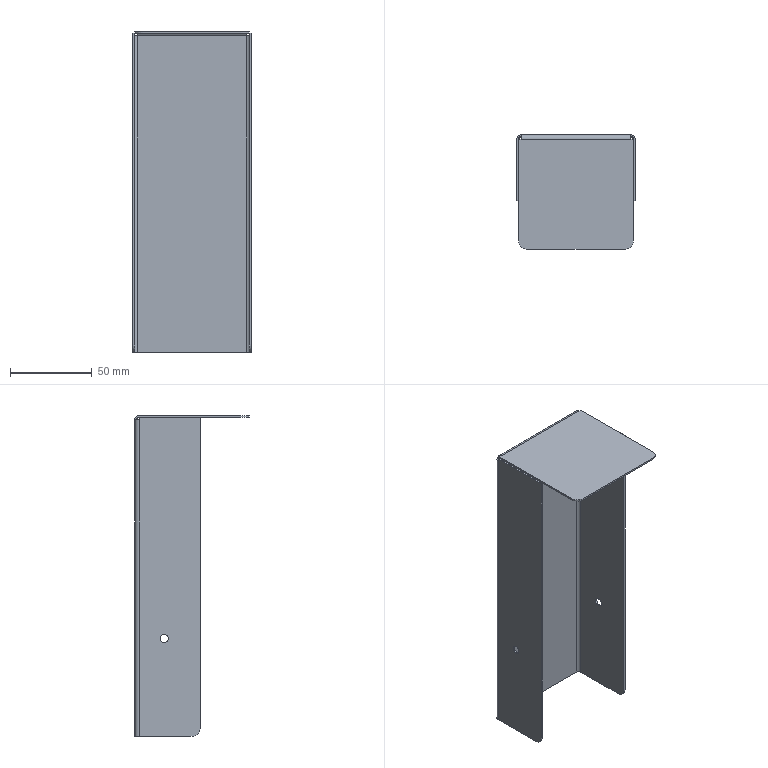Part | NX | 1 solid | 38 faces | box 72.4 x 70 x 196.5 mm | volume 33824 mm3 | plane 24 | cylinder 14 | commonest cylinder face diameters 5 x4 10 x4 3.2 x3 5.2 x3
STEP:
#1=CARTESIAN_POINT('',(-126.2,177.2,177.629));
#2=VERTEX_POINT('',#1);
#3=CARTESIAN_POINT('',(-126.2,214.6,177.629));
#4=VERTEX_POINT('',#3);
#5=CARTESIAN_POINT('',(-126.2,216.2,177.629));
#6=DIRECTION('',(0.,1.,0.));
#7=VECTOR('',#6,1000.);
#8=LINE('',#5,#7);
#9=EDGE_CURVE('',#2,#4,#8,.T.);
#10=ORIENTED_EDGE('',*,*,#9,.T.);
#11=CARTESIAN_POINT('',(-126.2,214.6,176.1));
#12=VERTEX_POINT('',#11);
#13=CARTESIAN_POINT('',(-126.2,214.6,70.628));
#14=DIRECTION('',(0.,0.,-1.));
#15=VECTOR('',#14,1000.);
#16=LINE('',#13,#15);
#17=EDGE_CURVE('',#4,#12,#16,.T.);
#18=ORIENTED_EDGE('',*,*,#17,.T.);
#19=CARTESIAN_POINT('',(-126.2,214.6,-17.8));
#20=VERTEX_POINT('',#19);
#21=CARTESIAN_POINT('',(-126.2,214.6,70.628));
#22=DIRECTION('',(0.,0.,-1.));
#23=VECTOR('',#22,1000.);
#24=LINE('',#21,#23);
#25=EDGE_CURVE('',#12,#20,#24,.T.);
#26=ORIENTED_EDGE('',*,*,#25,.T.);
#27=CARTESIAN_POINT('',(-126.2,182.2,-17.8));
#28=VERTEX_POINT('',#27);
#29=CARTESIAN_POINT('',(-126.2,177.2,-17.8));
#30=DIRECTION('',(0.,1.,0.));
#31=VECTOR('',#30,1000.);
#32=LINE('',#29,#31);
#33=EDGE_CURVE('',#28,#20,#32,.T.);
#34=ORIENTED_EDGE('',*,*,#33,.F.);
#35=CARTESIAN_POINT('',(-126.2,177.2,-12.8));
#36=VERTEX_POINT('',#35);
#37=CARTESIAN_POINT('',(-126.2,182.2,-12.8));
#38=DIRECTION('',(1.,0.,0.));
#39=DIRECTION('',(0.,0.,1.));
#40=AXIS2_PLACEMENT_3D('',#37,#38,#39);
#41=CIRCLE('',#40,5.);
#42=EDGE_CURVE('',#36,#28,#41,.T.);
#43=ORIENTED_EDGE('',*,*,#42,.F.);
#44=CARTESIAN_POINT('',(-126.2,177.2,70.628));
#45=DIRECTION('',(0.,0.,-1.));
#46=VECTOR('',#45,1000.);
#47=LINE('',#44,#46);
#48=EDGE_CURVE('',#2,#36,#47,.T.);
#49=ORIENTED_EDGE('',*,*,#48,.F.);
#50=EDGE_LOOP('',(#10,#18,#26,#34,#43,#49));
#51=FACE_BOUND('',#50,.T.);
#52=CARTESIAN_POINT('',(-126.2,201.7,42.2));
#53=VERTEX_POINT('',#52);
#54=CARTESIAN_POINT('',(-126.2,196.7,42.2));
#55=VERTEX_POINT('',#54);
#56=CARTESIAN_POINT('',(-126.2,199.2,42.2));
#57=DIRECTION('',(1.,0.,0.));
#58=DIRECTION('',(0.,-1.,0.));
#59=AXIS2_PLACEMENT_3D('',#56,#57,#58);
#60=CIRCLE('',#59,2.5);
#61=EDGE_CURVE('',#53,#55,#60,.T.);
#62=ORIENTED_EDGE('',*,*,#61,.T.);
#63=CARTESIAN_POINT('',(-126.2,199.2,42.2));
#64=DIRECTION('',(1.,0.,0.));
#65=DIRECTION('',(0.,-1.,0.));
#66=AXIS2_PLACEMENT_3D('',#63,#64,#65);
#67=CIRCLE('',#66,2.5);
#68=EDGE_CURVE('',#55,#53,#67,.T.);
#69=ORIENTED_EDGE('',*,*,#68,.T.);
#70=EDGE_LOOP('',(#62,#69));
#71=FACE_BOUND('',#70,.T.);
#72=CARTESIAN_POINT('',(-126.2,252.682,70.628));
#73=DIRECTION('',(-1.,0.,0.));
#74=DIRECTION('',(0.,0.,1.));
#75=AXIS2_PLACEMENT_3D('',#72,#73,#74);
#76=PLANE('',#75);
#77=ADVANCED_FACE('',(#51,#71),#76,.T.);
#78=CARTESIAN_POINT('',(-123.6,217.2,176.1));
#79=VERTEX_POINT('',#78);
#80=CARTESIAN_POINT('',(-123.6,217.2,-17.8));
#81=VERTEX_POINT('',#80);
#82=CARTESIAN_POINT('',(-123.6,217.2,70.628));
#83=DIRECTION('',(0.,0.,-1.));
#84=VECTOR('',#83,1000.);
#85=LINE('',#82,#84);
#86=EDGE_CURVE('',#79,#81,#85,.T.);
#87=ORIENTED_EDGE('',*,*,#86,.F.);
#88=CARTESIAN_POINT('',(-56.4,217.2,176.1));
#89=VERTEX_POINT('',#88);
#90=CARTESIAN_POINT('',(-88.618,217.2,176.1));
#91=DIRECTION('',(-1.,0.,0.));
#92=VECTOR('',#91,1000.);
#93=LINE('',#90,#92);
#94=EDGE_CURVE('',#89,#79,#93,.T.);
#95=ORIENTED_EDGE('',*,*,#94,.F.);
#96=CARTESIAN_POINT('',(-56.4,217.2,-17.8));
#97=VERTEX_POINT('',#96);
#98=CARTESIAN_POINT('',(-56.4,217.2,70.628));
#99=DIRECTION('',(0.,0.,1.));
#100=VECTOR('',#99,1000.);
#101=LINE('',#98,#100);
#102=EDGE_CURVE('',#97,#89,#101,.T.);
#103=ORIENTED_EDGE('',*,*,#102,.F.);
#104=CARTESIAN_POINT('',(-53.8,217.2,-17.8));
#105=DIRECTION('',(1.,0.,0.));
#106=VECTOR('',#105,1000.);
#107=LINE('',#104,#106);
#108=EDGE_CURVE('',#81,#97,#107,.T.);
#109=ORIENTED_EDGE('',*,*,#108,.F.);
#110=EDGE_LOOP('',(#87,#95,#103,#109));
#111=FACE_BOUND('',#110,.T.);
#112=CARTESIAN_POINT('',(-88.618,217.2,70.628));
#113=DIRECTION('',(0.,1.,0.));
#114=DIRECTION('',(0.,0.,-1.));
#115=AXIS2_PLACEMENT_3D('',#112,#113,#114);
#116=PLANE('',#115);
#117=ADVANCED_FACE('',(#111),#116,.T.);
#118=ORIENTED_EDGE('',*,*,#25,.F.);
#119=CARTESIAN_POINT('',(-123.6,214.6,176.1));
#120=DIRECTION('',(0.,0.,-1.));
#121=DIRECTION('',(-1.,0.,0.));
#122=AXIS2_PLACEMENT_3D('',#119,#120,#121);
#123=CIRCLE('',#122,2.6);
#124=EDGE_CURVE('',#12,#79,#123,.T.);
#125=ORIENTED_EDGE('',*,*,#124,.T.);
#126=ORIENTED_EDGE('',*,*,#86,.T.);
#127=CARTESIAN_POINT('',(-123.6,214.6,-17.8));
#128=DIRECTION('',(0.,0.,-1.));
#129=DIRECTION('',(-1.,0.,0.));
#130=AXIS2_PLACEMENT_3D('',#127,#128,#129);
#131=CIRCLE('',#130,2.6);
#132=EDGE_CURVE('',#20,#81,#131,.T.);
#133=ORIENTED_EDGE('',*,*,#132,.F.);
#134=EDGE_LOOP('',(#118,#125,#126,#133));
#135=FACE_BOUND('',#134,.T.);
#136=CARTESIAN_POINT('',(-123.6,214.6,-17.8));
#137=DIRECTION('',(0.,0.,-1.));
#138=DIRECTION('',(1.,0.,0.));
#139=AXIS2_PLACEMENT_3D('',#136,#137,#138);
#140=CYLINDRICAL_SURFACE('',#139,2.6);
#141=ADVANCED_FACE('',(#135),#140,.T.);
#142=CARTESIAN_POINT('',(-53.8,214.6,176.1));
#143=VERTEX_POINT('',#142);
#144=CARTESIAN_POINT('',(-53.8,214.6,177.629));
#145=VERTEX_POINT('',#144);
#146=CARTESIAN_POINT('',(-53.8,214.6,70.628));
#147=DIRECTION('',(0.,0.,1.));
#148=VECTOR('',#147,1000.);
#149=LINE('',#146,#148);
#150=EDGE_CURVE('',#143,#145,#149,.T.);
#151=ORIENTED_EDGE('',*,*,#150,.F.);
#152=CARTESIAN_POINT('',(-54.8,214.6,176.1));
#153=VERTEX_POINT('',#152);
#154=CARTESIAN_POINT('',(-53.8,214.6,176.1));
#155=DIRECTION('',(-1.,0.,0.));
#156=VECTOR('',#155,1000.);
#157=LINE('',#154,#156);
#158=EDGE_CURVE('',#143,#153,#157,.T.);
#159=ORIENTED_EDGE('',*,*,#158,.T.);
#160=CARTESIAN_POINT('',(-54.8,214.6,177.629));
#161=VERTEX_POINT('',#160);
#162=CARTESIAN_POINT('',(-54.8,214.6,70.628));
#163=DIRECTION('',(0.,0.,1.));
#164=VECTOR('',#163,1000.);
#165=LINE('',#162,#164);
#166=EDGE_CURVE('',#153,#161,#165,.T.);
#167=ORIENTED_EDGE('',*,*,#166,.T.);
#168=CARTESIAN_POINT('',(-54.8,214.6,177.629));
#169=DIRECTION('',(-1.,0.,0.));
#170=VECTOR('',#169,1000.);
#171=LINE('',#168,#170);
#172=EDGE_CURVE('',#145,#161,#171,.T.);
#173=ORIENTED_EDGE('',*,*,#172,.F.);
#174=EDGE_LOOP('',(#151,#159,#167,#173));
#175=FACE_BOUND('',#174,.T.);
#176=CARTESIAN_POINT('',(-53.8,214.6,176.1));
#177=DIRECTION('',(0.,1.,0.));
#178=DIRECTION('',(0.,0.,-1.));
#179=AXIS2_PLACEMENT_3D('',#176,#177,#178);
#180=PLANE('',#179);
#181=ADVANCED_FACE('',(#175),#180,.T.);
#182=CARTESIAN_POINT('',(-53.8,177.2,177.629));
#183=VERTEX_POINT('',#182);
#184=CARTESIAN_POINT('',(-53.8,216.2,177.629));
#185=DIRECTION('',(0.,-1.,0.));
#186=VECTOR('',#185,1000.);
#187=LINE('',#184,#186);
#188=EDGE_CURVE('',#145,#183,#187,.T.);
#189=ORIENTED_EDGE('',*,*,#188,.T.);
#190=CARTESIAN_POINT('',(-53.8,177.2,-12.8));
#191=VERTEX_POINT('',#190);
#192=CARTESIAN_POINT('',(-53.8,177.2,70.628));
#193=DIRECTION('',(0.,0.,1.));
#194=VECTOR('',#193,1000.);
#195=LINE('',#192,#194);
#196=EDGE_CURVE('',#191,#183,#195,.T.);
#197=ORIENTED_EDGE('',*,*,#196,.F.);
#198=CARTESIAN_POINT('',(-53.8,182.2,-17.8));
#199=VERTEX_POINT('',#198);
#200=CARTESIAN_POINT('',(-53.8,182.2,-12.8));
#201=DIRECTION('',(-1.,0.,0.));
#202=DIRECTION('',(0.,0.,-1.));
#203=AXIS2_PLACEMENT_3D('',#200,#201,#202);
#204=CIRCLE('',#203,5.);
#205=EDGE_CURVE('',#199,#191,#204,.T.);
#206=ORIENTED_EDGE('',*,*,#205,.F.);
#207=CARTESIAN_POINT('',(-53.8,214.6,-17.8));
#208=VERTEX_POINT('',#207);
#209=CARTESIAN_POINT('',(-53.8,215.1,-17.8));
#210=DIRECTION('',(0.,-1.,0.));
#211=VECTOR('',#210,1000.);
#212=LINE('',#209,#211);
#213=EDGE_CURVE('',#208,#199,#212,.T.);
#214=ORIENTED_EDGE('',*,*,#213,.F.);
#215=CARTESIAN_POINT('',(-53.8,214.6,70.628));
#216=DIRECTION('',(0.,0.,1.));
#217=VECTOR('',#216,1000.);
#218=LINE('',#215,#217);
#219=EDGE_CURVE('',#208,#143,#218,.T.);
#220=ORIENTED_EDGE('',*,*,#219,.T.);
#221=ORIENTED_EDGE('',*,*,#150,.T.);
#222=EDGE_LOOP('',(#189,#197,#206,#214,#220,#221));
#223=FACE_BOUND('',#222,.T.);
#224=CARTESIAN_POINT('',(-53.8,201.7,42.2));
#225=VERTEX_POINT('',#224);
#226=CARTESIAN_POINT('',(-53.8,196.7,42.2));
#227=VERTEX_POINT('',#226);
#228=CARTESIAN_POINT('',(-53.8,199.2,42.2));
#229=DIRECTION('',(1.,0.,0.));
#230=DIRECTION('',(0.,-1.,0.));
#231=AXIS2_PLACEMENT_3D('',#228,#229,#230);
#232=CIRCLE('',#231,2.5);
#233=EDGE_CURVE('',#225,#227,#232,.T.);
#234=ORIENTED_EDGE('',*,*,#233,.F.);
#235=CARTESIAN_POINT('',(-53.8,199.2,42.2));
#236=DIRECTION('',(1.,0.,0.));
#237=DIRECTION('',(0.,-1.,0.));
#238=AXIS2_PLACEMENT_3D('',#235,#236,#237);
#239=CIRCLE('',#238,2.5);
#240=EDGE_CURVE('',#227,#225,#239,.T.);
#241=ORIENTED_EDGE('',*,*,#240,.F.);
#242=EDGE_LOOP('',(#234,#241));
#243=FACE_BOUND('',#242,.T.);
#244=CARTESIAN_POINT('',(-53.8,249.918,70.628));
#245=DIRECTION('',(1.,0.,0.));
#246=DIRECTION('',(0.,1.,0.));
#247=AXIS2_PLACEMENT_3D('',#244,#245,#246);
#248=PLANE('',#247);
#249=ADVANCED_FACE('',(#223,#243),#248,.T.);
#250=CARTESIAN_POINT('',(-56.4,214.6,176.1));
#251=DIRECTION('',(0.,0.,-1.));
#252=DIRECTION('',(0.,1.,0.));
#253=AXIS2_PLACEMENT_3D('',#250,#251,#252);
#254=CIRCLE('',#253,2.6);
#255=EDGE_CURVE('',#89,#143,#254,.T.);
#256=ORIENTED_EDGE('',*,*,#255,.T.);
#257=ORIENTED_EDGE('',*,*,#219,.F.);
#258=CARTESIAN_POINT('',(-56.4,214.6,-17.8));
#259=DIRECTION('',(0.,0.,-1.));
#260=DIRECTION('',(0.,1.,0.));
#261=AXIS2_PLACEMENT_3D('',#258,#259,#260);
#262=CIRCLE('',#261,2.6);
#263=EDGE_CURVE('',#97,#208,#262,.T.);
#264=ORIENTED_EDGE('',*,*,#263,.F.);
#265=ORIENTED_EDGE('',*,*,#102,.T.);
#266=EDGE_LOOP('',(#256,#257,#264,#265));
#267=FACE_BOUND('',#266,.T.);
#268=CARTESIAN_POINT('',(-56.4,214.6,176.1));
#269=DIRECTION('',(0.,0.,1.));
#270=DIRECTION('',(-1.,0.,0.));
#271=AXIS2_PLACEMENT_3D('',#268,#269,#270);
#272=CYLINDRICAL_SURFACE('',#271,2.6);
#273=ADVANCED_FACE('',(#267),#272,.T.);
#274=CARTESIAN_POINT('',(-123.6,214.6,178.7));
#275=VERTEX_POINT('',#274);
#276=CARTESIAN_POINT('',(-123.6,214.6,176.1));
#277=DIRECTION('',(1.,0.,0.));
#278=DIRECTION('',(0.,1.,0.));
#279=AXIS2_PLACEMENT_3D('',#276,#277,#278);
#280=CIRCLE('',#279,2.6);
#281=EDGE_CURVE('',#79,#275,#280,.T.);
#282=ORIENTED_EDGE('',*,*,#281,.F.);
#283=CARTESIAN_POINT('',(-123.6,216.2,176.1));
#284=VERTEX_POINT('',#283);
#285=CARTESIAN_POINT('',(-123.6,217.2,176.1));
#286=DIRECTION('',(0.,-1.,0.));
#287=VECTOR('',#286,1000.);
#288=LINE('',#285,#287);
#289=EDGE_CURVE('',#79,#284,#288,.T.);
#290=ORIENTED_EDGE('',*,*,#289,.T.);
#291=CARTESIAN_POINT('',(-123.6,214.6,177.7));
#292=VERTEX_POINT('',#291);
#293=CARTESIAN_POINT('',(-123.6,214.6,176.1));
#294=DIRECTION('',(-1.,0.,0.));
#295=DIRECTION('',(0.,0.,1.));
#296=AXIS2_PLACEMENT_3D('',#293,#294,#295);
#297=CIRCLE('',#296,1.6);
#298=EDGE_CURVE('',#292,#284,#297,.T.);
#299=ORIENTED_EDGE('',*,*,#298,.F.);
#300=CARTESIAN_POINT('',(-123.6,214.6,178.7));
#301=DIRECTION('',(0.,0.,-1.));
#302=VECTOR('',#301,1000.);
#303=LINE('',#300,#302);
#304=EDGE_CURVE('',#275,#292,#303,.T.);
#305=ORIENTED_EDGE('',*,*,#304,.F.);
#306=EDGE_LOOP('',(#282,#290,#299,#305));
#307=FACE_BOUND('',#306,.T.);
#308=CARTESIAN_POINT('',(-123.6,214.6,176.1));
#309=DIRECTION('',(1.,0.,0.));
#310=DIRECTION('',(0.,1.,0.));
#311=AXIS2_PLACEMENT_3D('',#308,#309,#310);
#312=PLANE('',#311);
#313=ADVANCED_FACE('',(#307),#312,.F.);
#314=ORIENTED_EDGE('',*,*,#94,.T.);
#315=ORIENTED_EDGE('',*,*,#281,.T.);
#316=CARTESIAN_POINT('',(-56.4,214.6,178.7));
#317=VERTEX_POINT('',#316);
#318=CARTESIAN_POINT('',(-88.618,214.6,178.7));
#319=DIRECTION('',(-1.,0.,0.));
#320=VECTOR('',#319,1000.);
#321=LINE('',#318,#320);
#322=EDGE_CURVE('',#317,#275,#321,.T.);
#323=ORIENTED_EDGE('',*,*,#322,.F.);
#324=CARTESIAN_POINT('',(-56.4,214.6,176.1));
#325=DIRECTION('',(-1.,0.,0.));
#326=DIRECTION('',(0.,0.,1.));
#327=AXIS2_PLACEMENT_3D('',#324,#325,#326);
#328=CIRCLE('',#327,2.6);
#329=EDGE_CURVE('',#317,#89,#328,.T.);
#330=ORIENTED_EDGE('',*,*,#329,.T.);
#331=EDGE_LOOP('',(#314,#315,#323,#330));
#332=FACE_BOUND('',#331,.T.);
#333=CARTESIAN_POINT('',(-123.6,214.6,176.1));
#334=DIRECTION('',(-1.,0.,0.));
#335=DIRECTION('',(0.,0.,-1.));
#336=AXIS2_PLACEMENT_3D('',#333,#334,#335);
#337=CYLINDRICAL_SURFACE('',#336,2.6);
#338=ADVANCED_FACE('',(#332),#337,.T.);
#339=ORIENTED_EDGE('',*,*,#322,.T.);
#340=CARTESIAN_POINT('',(-125.129,214.6,178.7));
#341=VERTEX_POINT('',#340);
#342=CARTESIAN_POINT('',(-88.618,214.6,178.7));
#343=DIRECTION('',(-1.,0.,0.));
#344=VECTOR('',#343,1000.);
#345=LINE('',#342,#344);
#346=EDGE_CURVE('',#275,#341,#345,.T.);
#347=ORIENTED_EDGE('',*,*,#346,.T.);
#348=CARTESIAN_POINT('',(-125.129,152.2,178.7));
#349=VERTEX_POINT('',#348);
#350=CARTESIAN_POINT('',(-125.129,216.2,178.7));
#351=DIRECTION('',(0.,1.,0.));
#352=VECTOR('',#351,1000.);
#353=LINE('',#350,#352);
#354=EDGE_CURVE('',#349,#341,#353,.T.);
#355=ORIENTED_EDGE('',*,*,#354,.F.);
#356=CARTESIAN_POINT('',(-120.129,147.2,178.7));
#357=VERTEX_POINT('',#356);
#358=CARTESIAN_POINT('',(-120.129,152.2,178.7));
#359=DIRECTION('',(0.,0.,1.));
#360=DIRECTION('',(-1.,0.,0.));
#361=AXIS2_PLACEMENT_3D('',#358,#359,#360);
#362=CIRCLE('',#361,5.);
#363=EDGE_CURVE('',#349,#357,#362,.T.);
#364=ORIENTED_EDGE('',*,*,#363,.T.);
#365=CARTESIAN_POINT('',(-59.871,147.2,178.7));
#366=VERTEX_POINT('',#365);
#367=CARTESIAN_POINT('',(-88.618,147.2,178.7));
#368=DIRECTION('',(1.,0.,0.));
#369=VECTOR('',#368,1000.);
#370=LINE('',#367,#369);
#371=EDGE_CURVE('',#357,#366,#370,.T.);
#372=ORIENTED_EDGE('',*,*,#371,.T.);
#373=CARTESIAN_POINT('',(-54.871,152.2,178.7));
#374=VERTEX_POINT('',#373);
#375=CARTESIAN_POINT('',(-59.871,152.2,178.7));
#376=DIRECTION('',(0.,0.,-1.));
#377=DIRECTION('',(1.,0.,0.));
#378=AXIS2_PLACEMENT_3D('',#375,#376,#377);
#379=CIRCLE('',#378,5.);
#380=EDGE_CURVE('',#374,#366,#379,.T.);
#381=ORIENTED_EDGE('',*,*,#380,.F.);
#382=CARTESIAN_POINT('',(-54.871,214.6,178.7));
#383=VERTEX_POINT('',#382);
#384=CARTESIAN_POINT('',(-54.871,216.2,178.7));
#385=DIRECTION('',(0.,-1.,0.));
#386=VECTOR('',#385,1000.);
#387=LINE('',#384,#386);
#388=EDGE_CURVE('',#383,#374,#387,.T.);
#389=ORIENTED_EDGE('',*,*,#388,.F.);
#390=CARTESIAN_POINT('',(-88.618,214.6,178.7));
#391=DIRECTION('',(-1.,0.,0.));
#392=VECTOR('',#391,1000.);
#393=LINE('',#390,#392);
#394=EDGE_CURVE('',#383,#317,#393,.T.);
#395=ORIENTED_EDGE('',*,*,#394,.T.);
#396=EDGE_LOOP('',(#339,#347,#355,#364,#372,#381,#389,#395));
#397=FACE_BOUND('',#396,.T.);
#398=CARTESIAN_POINT('',(-88.618,323.172,178.7));
#399=DIRECTION('',(0.,0.,1.));
#400=DIRECTION('',(0.,-1.,0.));
#401=AXIS2_PLACEMENT_3D('',#398,#399,#400);
#402=PLANE('',#401);
#403=ADVANCED_FACE('',(#397),#402,.T.);
#404=ORIENTED_EDGE('',*,*,#48,.T.);
#405=CARTESIAN_POINT('',(-125.2,177.2,-12.8));
#406=VERTEX_POINT('',#405);
#407=CARTESIAN_POINT('',(-88.618,177.2,-12.8));
#408=DIRECTION('',(1.,0.,0.));
#409=VECTOR('',#408,1000.);
#410=LINE('',#407,#409);
#411=EDGE_CURVE('',#36,#406,#410,.T.);
#412=ORIENTED_EDGE('',*,*,#411,.T.);
#413=CARTESIAN_POINT('',(-125.2,177.2,177.629));
#414=VERTEX_POINT('',#413);
#415=CARTESIAN_POINT('',(-125.2,177.2,70.628));
#416=DIRECTION('',(0.,0.,-1.));
#417=VECTOR('',#416,1000.);
#418=LINE('',#415,#417);
#419=EDGE_CURVE('',#414,#406,#418,.T.);
#420=ORIENTED_EDGE('',*,*,#419,.F.);
#421=CARTESIAN_POINT('',(-88.618,177.2,177.629));
#422=DIRECTION('',(-1.,0.,0.));
#423=VECTOR('',#422,1000.);
#424=LINE('',#421,#423);
#425=EDGE_CURVE('',#414,#2,#424,.T.);
#426=ORIENTED_EDGE('',*,*,#425,.T.);
#427=EDGE_LOOP('',(#404,#412,#420,#426));
#428=FACE_BOUND('',#427,.T.);
#429=CARTESIAN_POINT('',(-126.2,177.2,-17.8));
#430=DIRECTION('',(0.,-1.,0.));
#431=DIRECTION('',(0.,0.,-1.));
#432=AXIS2_PLACEMENT_3D('',#429,#430,#431);
#433=PLANE('',#432);
#434=ADVANCED_FACE('',(#428),#433,.T.);
#435=CARTESIAN_POINT('',(-125.2,214.6,176.1));
#436=VERTEX_POINT('',#435);
#437=CARTESIAN_POINT('',(-125.2,214.6,-17.8));
#438=VERTEX_POINT('',#437);
#439=CARTESIAN_POINT('',(-125.2,214.6,70.628));
#440=DIRECTION('',(0.,0.,-1.));
#441=VECTOR('',#440,1000.);
#442=LINE('',#439,#441);
#443=EDGE_CURVE('',#436,#438,#442,.T.);
#444=ORIENTED_EDGE('',*,*,#443,.F.);
#445=CARTESIAN_POINT('',(-125.2,214.6,177.629));
#446=VERTEX_POINT('',#445);
#447=CARTESIAN_POINT('',(-125.2,214.6,70.628));
#448=DIRECTION('',(0.,0.,-1.));
#449=VECTOR('',#448,1000.);
#450=LINE('',#447,#449);
#451=EDGE_CURVE('',#446,#436,#450,.T.);
#452=ORIENTED_EDGE('',*,*,#451,.F.);
#453=CARTESIAN_POINT('',(-125.2,216.2,177.629));
#454=DIRECTION('',(0.,1.,0.));
#455=VECTOR('',#454,1000.);
#456=LINE('',#453,#455);
#457=EDGE_CURVE('',#414,#446,#456,.T.);
#458=ORIENTED_EDGE('',*,*,#457,.F.);
#459=ORIENTED_EDGE('',*,*,#419,.T.);
#460=CARTESIAN_POINT('',(-125.2,182.2,-17.8));
#461=VERTEX_POINT('',#460);
#462=CARTESIAN_POINT('',(-125.2,182.2,-12.8));
#463=DIRECTION('',(1.,0.,0.));
#464=DIRECTION('',(0.,0.,1.));
#465=AXIS2_PLACEMENT_3D('',#462,#463,#464);
#466=CIRCLE('',#465,5.);
#467=EDGE_CURVE('',#406,#461,#466,.T.);
#468=ORIENTED_EDGE('',*,*,#467,.T.);
#469=CARTESIAN_POINT('',(-125.2,177.2,-17.8));
#470=DIRECTION('',(0.,1.,0.));
#471=VECTOR('',#470,1000.);
#472=LINE('',#469,#471);
#473=EDGE_CURVE('',#461,#438,#472,.T.);
#474=ORIENTED_EDGE('',*,*,#473,.T.);
#475=EDGE_LOOP('',(#444,#452,#458,#459,#468,#474));
#476=FACE_BOUND('',#475,.T.);
#477=CARTESIAN_POINT('',(-125.2,201.7,42.2));
#478=VERTEX_POINT('',#477);
#479=CARTESIAN_POINT('',(-125.2,196.7,42.2));
#480=VERTEX_POINT('',#479);
#481=CARTESIAN_POINT('',(-125.2,199.2,42.2));
#482=DIRECTION('',(1.,0.,0.));
#483=DIRECTION('',(0.,-1.,0.));
#484=AXIS2_PLACEMENT_3D('',#481,#482,#483);
#485=CIRCLE('',#484,2.5);
#486=EDGE_CURVE('',#478,#480,#485,.T.);
#487=ORIENTED_EDGE('',*,*,#486,.F.);
#488=CARTESIAN_POINT('',(-125.2,199.2,42.2));
#489=DIRECTION('',(1.,0.,0.));
#490=DIRECTION('',(0.,-1.,0.));
#491=AXIS2_PLACEMENT_3D('',#488,#489,#490);
#492=CIRCLE('',#491,2.5);
#493=EDGE_CURVE('',#480,#478,#492,.T.);
#494=ORIENTED_EDGE('',*,*,#493,.F.);
#495=EDGE_LOOP('',(#487,#494));
#496=FACE_BOUND('',#495,.T.);
#497=CARTESIAN_POINT('',(-125.2,215.1,175.2));
#498=DIRECTION('',(-1.,0.,0.));
#499=DIRECTION('',(0.,0.,1.));
#500=AXIS2_PLACEMENT_3D('',#497,#498,#499);
#501=PLANE('',#500);
#502=ADVANCED_FACE('',(#476,#496),#501,.F.);
#503=CARTESIAN_POINT('',(-123.6,216.2,-17.8));
#504=VERTEX_POINT('',#503);
#505=CARTESIAN_POINT('',(-123.6,216.2,70.628));
#506=DIRECTION('',(0.,0.,-1.));
#507=VECTOR('',#506,1000.);
#508=LINE('',#505,#507);
#509=EDGE_CURVE('',#284,#504,#508,.T.);
#510=ORIENTED_EDGE('',*,*,#509,.F.);
#511=CARTESIAN_POINT('',(-123.6,214.6,176.1));
#512=DIRECTION('',(0.,0.,1.));
#513=DIRECTION('',(0.,1.,0.));
#514=AXIS2_PLACEMENT_3D('',#511,#512,#513);
#515=CIRCLE('',#514,1.6);
#516=EDGE_CURVE('',#284,#436,#515,.T.);
#517=ORIENTED_EDGE('',*,*,#516,.T.);
#518=ORIENTED_EDGE('',*,*,#443,.T.);
#519=CARTESIAN_POINT('',(-123.6,214.6,-17.8));
#520=DIRECTION('',(0.,0.,-1.));
#521=DIRECTION('',(-1.,0.,0.));
#522=AXIS2_PLACEMENT_3D('',#519,#520,#521);
#523=CIRCLE('',#522,1.6);
#524=EDGE_CURVE('',#438,#504,#523,.T.);
#525=ORIENTED_EDGE('',*,*,#524,.T.);
#526=EDGE_LOOP('',(#510,#517,#518,#525));
#527=FACE_BOUND('',#526,.T.);
#528=CARTESIAN_POINT('',(-123.6,214.6,-17.8));
#529=DIRECTION('',(0.,0.,-1.));
#530=DIRECTION('',(1.,0.,0.));
#531=AXIS2_PLACEMENT_3D('',#528,#529,#530);
#532=CYLINDRICAL_SURFACE('',#531,1.6);
#533=ADVANCED_FACE('',(#527),#532,.F.);
#534=ORIENTED_EDGE('',*,*,#61,.F.);
#535=CARTESIAN_POINT('',(-133.44,201.7,42.2));
#536=DIRECTION('',(1.,0.,0.));
#537=VECTOR('',#536,1000.);
#538=LINE('',#535,#537);
#539=EDGE_CURVE('',#478,#53,#538,.F.);
#540=ORIENTED_EDGE('',*,*,#539,.F.);
#541=ORIENTED_EDGE('',*,*,#486,.T.);
#542=CARTESIAN_POINT('',(-133.44,196.7,42.2));
#543=DIRECTION('',(1.,0.,0.));
#544=VECTOR('',#543,1000.);
#545=LINE('',#542,#544);
#546=EDGE_CURVE('',#480,#55,#545,.F.);
#547=ORIENTED_EDGE('',*,*,#546,.T.);
#548=EDGE_LOOP('',(#534,#540,#541,#547));
#549=FACE_BOUND('',#548,.T.);
#550=CARTESIAN_POINT('',(-133.44,199.2,42.2));
#551=DIRECTION('',(1.,0.,0.));
#552=DIRECTION('',(0.,-1.,0.));
#553=AXIS2_PLACEMENT_3D('',#550,#551,#552);
#554=CYLINDRICAL_SURFACE('',#553,2.5);
#555=ADVANCED_FACE('',(#549),#554,.F.);
#556=ORIENTED_EDGE('',*,*,#546,.F.);
#557=ORIENTED_EDGE('',*,*,#493,.T.);
#558=ORIENTED_EDGE('',*,*,#539,.T.);
#559=ORIENTED_EDGE('',*,*,#68,.F.);
#560=EDGE_LOOP('',(#556,#557,#558,#559));
#561=FACE_BOUND('',#560,.T.);
#562=CARTESIAN_POINT('',(-133.44,199.2,42.2));
#563=DIRECTION('',(1.,0.,0.));
#564=DIRECTION('',(0.,-1.,0.));
#565=AXIS2_PLACEMENT_3D('',#562,#563,#564);
#566=CYLINDRICAL_SURFACE('',#565,2.5);
#567=ADVANCED_FACE('',(#561),#566,.F.);
#568=CARTESIAN_POINT('',(-54.8,214.6,-17.8));
#569=VERTEX_POINT('',#568);
#570=CARTESIAN_POINT('',(-54.8,182.2,-17.8));
#571=VERTEX_POINT('',#570);
#572=CARTESIAN_POINT('',(-54.8,215.1,-17.8));
#573=DIRECTION('',(0.,-1.,0.));
#574=VECTOR('',#573,1000.);
#575=LINE('',#572,#574);
#576=EDGE_CURVE('',#569,#571,#575,.T.);
#577=ORIENTED_EDGE('',*,*,#576,.T.);
#578=CARTESIAN_POINT('',(-54.8,177.2,-12.8));
#579=VERTEX_POINT('',#578);
#580=CARTESIAN_POINT('',(-54.8,182.2,-12.8));
#581=DIRECTION('',(-1.,0.,0.));
#582=DIRECTION('',(0.,0.,-1.));
#583=AXIS2_PLACEMENT_3D('',#580,#581,#582);
#584=CIRCLE('',#583,5.);
#585=EDGE_CURVE('',#571,#579,#584,.T.);
#586=ORIENTED_EDGE('',*,*,#585,.T.);
#587=CARTESIAN_POINT('',(-54.8,177.2,177.629));
#588=VERTEX_POINT('',#587);
#589=CARTESIAN_POINT('',(-54.8,177.2,70.628));
#590=DIRECTION('',(0.,0.,1.));
#591=VECTOR('',#590,1000.);
#592=LINE('',#589,#591);
#593=EDGE_CURVE('',#579,#588,#592,.T.);
#594=ORIENTED_EDGE('',*,*,#593,.T.);
#595=CARTESIAN_POINT('',(-54.8,216.2,177.629));
#596=DIRECTION('',(0.,-1.,0.));
#597=VECTOR('',#596,1000.);
#598=LINE('',#595,#597);
#599=EDGE_CURVE('',#161,#588,#598,.T.);
#600=ORIENTED_EDGE('',*,*,#599,.F.);
#601=ORIENTED_EDGE('',*,*,#166,.F.);
#602=CARTESIAN_POINT('',(-54.8,214.6,70.628));
#603=DIRECTION('',(0.,0.,1.));
#604=VECTOR('',#603,1000.);
#605=LINE('',#602,#604);
#606=EDGE_CURVE('',#569,#153,#605,.T.);
#607=ORIENTED_EDGE('',*,*,#606,.F.);
#608=EDGE_LOOP('',(#577,#586,#594,#600,#601,#607));
#609=FACE_BOUND('',#608,.T.);
#610=CARTESIAN_POINT('',(-54.8,201.7,42.2));
#611=VERTEX_POINT('',#610);
#612=CARTESIAN_POINT('',(-54.8,196.7,42.2));
#613=VERTEX_POINT('',#612);
#614=CARTESIAN_POINT('',(-54.8,199.2,42.2));
#615=DIRECTION('',(1.,0.,0.));
#616=DIRECTION('',(0.,-1.,0.));
#617=AXIS2_PLACEMENT_3D('',#614,#615,#616);
#618=CIRCLE('',#617,2.5);
#619=EDGE_CURVE('',#611,#613,#618,.T.);
#620=ORIENTED_EDGE('',*,*,#619,.T.);
#621=CARTESIAN_POINT('',(-54.8,199.2,42.2));
#622=DIRECTION('',(1.,0.,0.));
#623=DIRECTION('',(0.,-1.,0.));
#624=AXIS2_PLACEMENT_3D('',#621,#622,#623);
#625=CIRCLE('',#624,2.5);
#626=EDGE_CURVE('',#613,#611,#625,.T.);
#627=ORIENTED_EDGE('',*,*,#626,.T.);
#628=EDGE_LOOP('',(#620,#627));
#629=FACE_BOUND('',#628,.T.);
#630=CARTESIAN_POINT('',(-54.8,215.1,-17.8));
#631=DIRECTION('',(1.,0.,0.));
#632=DIRECTION('',(0.,1.,0.));
#633=AXIS2_PLACEMENT_3D('',#630,#631,#632);
#634=PLANE('',#633);
#635=ADVANCED_FACE('',(#609,#629),#634,.F.);
#636=ORIENTED_EDGE('',*,*,#196,.T.);
#637=CARTESIAN_POINT('',(-88.618,177.2,177.629));
#638=DIRECTION('',(-1.,0.,0.));
#639=VECTOR('',#638,1000.);
#640=LINE('',#637,#639);
#641=EDGE_CURVE('',#183,#588,#640,.T.);
#642=ORIENTED_EDGE('',*,*,#641,.T.);
#643=ORIENTED_EDGE('',*,*,#593,.F.);
#644=CARTESIAN_POINT('',(-88.618,177.2,-12.8));
#645=DIRECTION('',(-1.,0.,0.));
#646=VECTOR('',#645,1000.);
#647=LINE('',#644,#646);
#648=EDGE_CURVE('',#191,#579,#647,.T.);
#649=ORIENTED_EDGE('',*,*,#648,.F.);
#650=EDGE_LOOP('',(#636,#642,#643,#649));
#651=FACE_BOUND('',#650,.T.);
#652=CARTESIAN_POINT('',(-53.8,177.2,175.2));
#653=DIRECTION('',(0.,-1.,0.));
#654=DIRECTION('',(0.,0.,-1.));
#655=AXIS2_PLACEMENT_3D('',#652,#653,#654);
#656=PLANE('',#655);
#657=ADVANCED_FACE('',(#651),#656,.T.);
#658=CARTESIAN_POINT('',(-125.2,214.6,177.629));
#659=DIRECTION('',(-1.,0.,0.));
#660=VECTOR('',#659,1000.);
#661=LINE('',#658,#660);
#662=EDGE_CURVE('',#446,#4,#661,.T.);
#663=ORIENTED_EDGE('',*,*,#662,.T.);
#664=ORIENTED_EDGE('',*,*,#9,.F.);
#665=ORIENTED_EDGE('',*,*,#425,.F.);
#666=ORIENTED_EDGE('',*,*,#457,.T.);
#667=EDGE_LOOP('',(#663,#664,#665,#666));
#668=FACE_BOUND('',#667,.T.);
#669=CARTESIAN_POINT('',(-125.2,195.9,177.629));
#670=DIRECTION('',(0.,0.,1.));
#671=DIRECTION('',(1.,0.,0.));
#672=AXIS2_PLACEMENT_3D('',#669,#670,#671);
#673=PLANE('',#672);
#674=ADVANCED_FACE('',(#668),#673,.T.);
#675=ORIENTED_EDGE('',*,*,#599,.T.);
#676=ORIENTED_EDGE('',*,*,#641,.F.);
#677=ORIENTED_EDGE('',*,*,#188,.F.);
#678=ORIENTED_EDGE('',*,*,#172,.T.);
#679=EDGE_LOOP('',(#675,#676,#677,#678));
#680=FACE_BOUND('',#679,.T.);
#681=CARTESIAN_POINT('',(-54.8,195.9,177.629));
#682=DIRECTION('',(0.,0.,1.));
#683=DIRECTION('',(1.,0.,0.));
#684=AXIS2_PLACEMENT_3D('',#681,#682,#683);
#685=PLANE('',#684);
#686=ADVANCED_FACE('',(#680),#685,.T.);
#687=CARTESIAN_POINT('',(-56.4,214.6,177.7));
#688=VERTEX_POINT('',#687);
#689=CARTESIAN_POINT('',(-56.4,216.2,176.1));
#690=VERTEX_POINT('',#689);
#691=CARTESIAN_POINT('',(-56.4,214.6,176.1));
#692=DIRECTION('',(-1.,0.,0.));
#693=DIRECTION('',(0.,0.,1.));
#694=AXIS2_PLACEMENT_3D('',#691,#692,#693);
#695=CIRCLE('',#694,1.6);
#696=EDGE_CURVE('',#688,#690,#695,.T.);
#697=ORIENTED_EDGE('',*,*,#696,.F.);
#698=CARTESIAN_POINT('',(-88.618,214.6,177.7));
#699=DIRECTION('',(-1.,0.,0.));
#700=VECTOR('',#699,1000.);
#701=LINE('',#698,#700);
#702=EDGE_CURVE('',#688,#292,#701,.T.);
#703=ORIENTED_EDGE('',*,*,#702,.T.);
#704=ORIENTED_EDGE('',*,*,#298,.T.);
#705=CARTESIAN_POINT('',(-88.618,216.2,176.1));
#706=DIRECTION('',(-1.,0.,0.));
#707=VECTOR('',#706,1000.);
#708=LINE('',#705,#707);
#709=EDGE_CURVE('',#690,#284,#708,.T.);
#710=ORIENTED_EDGE('',*,*,#709,.F.);
#711=EDGE_LOOP('',(#697,#703,#704,#710));
#712=FACE_BOUND('',#711,.T.);
#713=CARTESIAN_POINT('',(-123.6,214.6,176.1));
#714=DIRECTION('',(-1.,0.,0.));
#715=DIRECTION('',(0.,0.,-1.));
#716=AXIS2_PLACEMENT_3D('',#713,#714,#715);
#717=CYLINDRICAL_SURFACE('',#716,1.6);
#718=ADVANCED_FACE('',(#712),#717,.F.);
#719=CARTESIAN_POINT('',(-56.4,214.6,176.1));
#720=DIRECTION('',(0.,0.,1.));
#721=DIRECTION('',(1.,0.,0.));
#722=AXIS2_PLACEMENT_3D('',#719,#720,#721);
#723=CIRCLE('',#722,1.6);
#724=EDGE_CURVE('',#153,#690,#723,.T.);
#725=ORIENTED_EDGE('',*,*,#724,.T.);
#726=CARTESIAN_POINT('',(-56.4,216.2,-17.8));
#727=VERTEX_POINT('',#726);
#728=CARTESIAN_POINT('',(-56.4,216.2,70.628));
#729=DIRECTION('',(0.,0.,1.));
#730=VECTOR('',#729,1000.);
#731=LINE('',#728,#730);
#732=EDGE_CURVE('',#727,#690,#731,.T.);
#733=ORIENTED_EDGE('',*,*,#732,.F.);
#734=CARTESIAN_POINT('',(-56.4,214.6,-17.8));
#735=DIRECTION('',(0.,0.,-1.));
#736=DIRECTION('',(0.,1.,0.));
#737=AXIS2_PLACEMENT_3D('',#734,#735,#736);
#738=CIRCLE('',#737,1.6);
#739=EDGE_CURVE('',#727,#569,#738,.T.);
#740=ORIENTED_EDGE('',*,*,#739,.T.);
#741=ORIENTED_EDGE('',*,*,#606,.T.);
#742=EDGE_LOOP('',(#725,#733,#740,#741));
#743=FACE_BOUND('',#742,.T.);
#744=CARTESIAN_POINT('',(-56.4,214.6,176.1));
#745=DIRECTION('',(0.,0.,1.));
#746=DIRECTION('',(-1.,0.,0.));
#747=AXIS2_PLACEMENT_3D('',#744,#745,#746);
#748=CYLINDRICAL_SURFACE('',#747,1.6);
#749=ADVANCED_FACE('',(#743),#748,.F.);
#750=CARTESIAN_POINT('',(-88.618,182.2,-17.8));
#751=DIRECTION('',(-1.,0.,0.));
#752=VECTOR('',#751,1000.);
#753=LINE('',#750,#752);
#754=EDGE_CURVE('',#199,#571,#753,.T.);
#755=ORIENTED_EDGE('',*,*,#754,.T.);
#756=ORIENTED_EDGE('',*,*,#576,.F.);
#757=ORIENTED_EDGE('',*,*,#739,.F.);
#758=CARTESIAN_POINT('',(-53.8,216.2,-17.8));
#759=DIRECTION('',(1.,0.,0.));
#760=VECTOR('',#759,1000.);
#761=LINE('',#758,#760);
#762=EDGE_CURVE('',#504,#727,#761,.T.);
#763=ORIENTED_EDGE('',*,*,#762,.F.);
#764=ORIENTED_EDGE('',*,*,#524,.F.);
#765=ORIENTED_EDGE('',*,*,#473,.F.);
#766=CARTESIAN_POINT('',(-88.618,182.2,-17.8));
#767=DIRECTION('',(1.,0.,0.));
#768=VECTOR('',#767,1000.);
#769=LINE('',#766,#768);
#770=EDGE_CURVE('',#28,#461,#769,.T.);
#771=ORIENTED_EDGE('',*,*,#770,.F.);
#772=ORIENTED_EDGE('',*,*,#33,.T.);
#773=ORIENTED_EDGE('',*,*,#132,.T.);
#774=ORIENTED_EDGE('',*,*,#108,.T.);
#775=ORIENTED_EDGE('',*,*,#263,.T.);
#776=ORIENTED_EDGE('',*,*,#213,.T.);
#777=EDGE_LOOP('',(#755,#756,#757,#763,#764,#765,#771,#772,#773,#774,#775,#776));
#778=FACE_BOUND('',#777,.T.);
#779=CARTESIAN_POINT('',(-15.9,217.2,-17.8));
#780=DIRECTION('',(0.,0.,-1.));
#781=DIRECTION('',(0.,-1.,0.));
#782=AXIS2_PLACEMENT_3D('',#779,#780,#781);
#783=PLANE('',#782);
#784=ADVANCED_FACE('',(#778),#783,.T.);
#785=ORIENTED_EDGE('',*,*,#255,.F.);
#786=CARTESIAN_POINT('',(-56.4,217.2,176.1));
#787=DIRECTION('',(0.,-1.,0.));
#788=VECTOR('',#787,1000.);
#789=LINE('',#786,#788);
#790=EDGE_CURVE('',#89,#690,#789,.T.);
#791=ORIENTED_EDGE('',*,*,#790,.T.);
#792=ORIENTED_EDGE('',*,*,#724,.F.);
#793=ORIENTED_EDGE('',*,*,#158,.F.);
#794=EDGE_LOOP('',(#785,#791,#792,#793));
#795=FACE_BOUND('',#794,.T.);
#796=CARTESIAN_POINT('',(-56.4,214.6,176.1));
#797=DIRECTION('',(0.,0.,-1.));
#798=DIRECTION('',(-1.,0.,0.));
#799=AXIS2_PLACEMENT_3D('',#796,#797,#798);
#800=PLANE('',#799);
#801=ADVANCED_FACE('',(#795),#800,.F.);
#802=CARTESIAN_POINT('',(-125.129,214.6,177.7));
#803=VERTEX_POINT('',#802);
#804=CARTESIAN_POINT('',(-125.129,214.6,177.7));
#805=DIRECTION('',(0.,0.,-1.));
#806=VECTOR('',#805,1000.);
#807=LINE('',#804,#806);
#808=EDGE_CURVE('',#341,#803,#807,.T.);
#809=ORIENTED_EDGE('',*,*,#808,.F.);
#810=ORIENTED_EDGE('',*,*,#346,.F.);
#811=ORIENTED_EDGE('',*,*,#304,.T.);
#812=CARTESIAN_POINT('',(-88.618,214.6,177.7));
#813=DIRECTION('',(-1.,0.,0.));
#814=VECTOR('',#813,1000.);
#815=LINE('',#812,#814);
#816=EDGE_CURVE('',#292,#803,#815,.T.);
#817=ORIENTED_EDGE('',*,*,#816,.T.);
#818=EDGE_LOOP('',(#809,#810,#811,#817));
#819=FACE_BOUND('',#818,.T.);
#820=CARTESIAN_POINT('',(-123.6,214.6,178.7));
#821=DIRECTION('',(0.,1.,0.));
#822=DIRECTION('',(0.,0.,-1.));
#823=AXIS2_PLACEMENT_3D('',#820,#821,#822);
#824=PLANE('',#823);
#825=ADVANCED_FACE('',(#819),#824,.T.);
#826=ORIENTED_EDGE('',*,*,#124,.F.);
#827=CARTESIAN_POINT('',(-126.2,214.6,176.1));
#828=DIRECTION('',(1.,0.,0.));
#829=VECTOR('',#828,1000.);
#830=LINE('',#827,#829);
#831=EDGE_CURVE('',#12,#436,#830,.T.);
#832=ORIENTED_EDGE('',*,*,#831,.T.);
#833=ORIENTED_EDGE('',*,*,#516,.F.);
#834=ORIENTED_EDGE('',*,*,#289,.F.);
#835=EDGE_LOOP('',(#826,#832,#833,#834));
#836=FACE_BOUND('',#835,.T.);
#837=CARTESIAN_POINT('',(-123.6,214.6,176.1));
#838=DIRECTION('',(0.,0.,-1.));
#839=DIRECTION('',(-1.,0.,0.));
#840=AXIS2_PLACEMENT_3D('',#837,#838,#839);
#841=PLANE('',#840);
#842=ADVANCED_FACE('',(#836),#841,.F.);
#843=ORIENTED_EDGE('',*,*,#709,.T.);
#844=ORIENTED_EDGE('',*,*,#509,.T.);
#845=ORIENTED_EDGE('',*,*,#762,.T.);
#846=ORIENTED_EDGE('',*,*,#732,.T.);
#847=EDGE_LOOP('',(#843,#844,#845,#846));
#848=FACE_BOUND('',#847,.T.);
#849=CARTESIAN_POINT('',(-53.8,216.2,-17.8));
#850=DIRECTION('',(0.,1.,0.));
#851=DIRECTION('',(0.,0.,-1.));
#852=AXIS2_PLACEMENT_3D('',#849,#850,#851);
#853=PLANE('',#852);
#854=ADVANCED_FACE('',(#848),#853,.F.);
#855=ORIENTED_EDGE('',*,*,#702,.F.);
#856=CARTESIAN_POINT('',(-54.871,214.6,177.7));
#857=VERTEX_POINT('',#856);
#858=CARTESIAN_POINT('',(-88.618,214.6,177.7));
#859=DIRECTION('',(-1.,0.,0.));
#860=VECTOR('',#859,1000.);
#861=LINE('',#858,#860);
#862=EDGE_CURVE('',#857,#688,#861,.T.);
#863=ORIENTED_EDGE('',*,*,#862,.F.);
#864=CARTESIAN_POINT('',(-54.871,152.2,177.7));
#865=VERTEX_POINT('',#864);
#866=CARTESIAN_POINT('',(-54.871,216.2,177.7));
#867=DIRECTION('',(0.,-1.,0.));
#868=VECTOR('',#867,1000.);
#869=LINE('',#866,#868);
#870=EDGE_CURVE('',#857,#865,#869,.T.);
#871=ORIENTED_EDGE('',*,*,#870,.T.);
#872=CARTESIAN_POINT('',(-59.871,147.2,177.7));
#873=VERTEX_POINT('',#872);
#874=CARTESIAN_POINT('',(-59.871,152.2,177.7));
#875=DIRECTION('',(0.,0.,-1.));
#876=DIRECTION('',(1.,0.,0.));
#877=AXIS2_PLACEMENT_3D('',#874,#875,#876);
#878=CIRCLE('',#877,5.);
#879=EDGE_CURVE('',#865,#873,#878,.T.);
#880=ORIENTED_EDGE('',*,*,#879,.T.);
#881=CARTESIAN_POINT('',(-120.129,147.2,177.7));
#882=VERTEX_POINT('',#881);
#883=CARTESIAN_POINT('',(-88.618,147.2,177.7));
#884=DIRECTION('',(1.,0.,0.));
#885=VECTOR('',#884,1000.);
#886=LINE('',#883,#885);
#887=EDGE_CURVE('',#882,#873,#886,.T.);
#888=ORIENTED_EDGE('',*,*,#887,.F.);
#889=CARTESIAN_POINT('',(-125.129,152.2,177.7));
#890=VERTEX_POINT('',#889);
#891=CARTESIAN_POINT('',(-120.129,152.2,177.7));
#892=DIRECTION('',(0.,0.,1.));
#893=DIRECTION('',(-1.,0.,0.));
#894=AXIS2_PLACEMENT_3D('',#891,#892,#893);
#895=CIRCLE('',#894,5.);
#896=EDGE_CURVE('',#890,#882,#895,.T.);
#897=ORIENTED_EDGE('',*,*,#896,.F.);
#898=CARTESIAN_POINT('',(-125.129,216.2,177.7));
#899=DIRECTION('',(0.,1.,0.));
#900=VECTOR('',#899,1000.);
#901=LINE('',#898,#900);
#902=EDGE_CURVE('',#890,#803,#901,.T.);
#903=ORIENTED_EDGE('',*,*,#902,.T.);
#904=ORIENTED_EDGE('',*,*,#816,.F.);
#905=EDGE_LOOP('',(#855,#863,#871,#880,#888,#897,#903,#904));
#906=FACE_BOUND('',#905,.T.);
#907=CARTESIAN_POINT('',(-53.8,411.6,177.7));
#908=DIRECTION('',(0.,0.,1.));
#909=DIRECTION('',(0.,-1.,0.));
#910=AXIS2_PLACEMENT_3D('',#907,#908,#909);
#911=PLANE('',#910);
#912=ADVANCED_FACE('',(#906),#911,.F.);
#913=ORIENTED_EDGE('',*,*,#770,.T.);
#914=ORIENTED_EDGE('',*,*,#467,.F.);
#915=ORIENTED_EDGE('',*,*,#411,.F.);
#916=ORIENTED_EDGE('',*,*,#42,.T.);
#917=EDGE_LOOP('',(#913,#914,#915,#916));
#918=FACE_BOUND('',#917,.T.);
#919=CARTESIAN_POINT('',(-88.618,182.2,-12.8));
#920=DIRECTION('',(1.,0.,0.));
#921=DIRECTION('',(0.,0.,1.));
#922=AXIS2_PLACEMENT_3D('',#919,#920,#921);
#923=CYLINDRICAL_SURFACE('',#922,5.);
#924=ADVANCED_FACE('',(#918),#923,.T.);
#925=ORIENTED_EDGE('',*,*,#754,.F.);
#926=ORIENTED_EDGE('',*,*,#205,.T.);
#927=ORIENTED_EDGE('',*,*,#648,.T.);
#928=ORIENTED_EDGE('',*,*,#585,.F.);
#929=EDGE_LOOP('',(#925,#926,#927,#928));
#930=FACE_BOUND('',#929,.T.);
#931=CARTESIAN_POINT('',(-88.618,182.2,-12.8));
#932=DIRECTION('',(-1.,0.,0.));
#933=DIRECTION('',(0.,0.,-1.));
#934=AXIS2_PLACEMENT_3D('',#931,#932,#933);
#935=CYLINDRICAL_SURFACE('',#934,5.);
#936=ADVANCED_FACE('',(#930),#935,.T.);
#937=ORIENTED_EDGE('',*,*,#619,.F.);
#938=CARTESIAN_POINT('',(-133.44,201.7,42.2));
#939=DIRECTION('',(1.,0.,0.));
#940=VECTOR('',#939,1000.);
#941=LINE('',#938,#940);
#942=EDGE_CURVE('',#225,#611,#941,.F.);
#943=ORIENTED_EDGE('',*,*,#942,.F.);
#944=ORIENTED_EDGE('',*,*,#233,.T.);
#945=CARTESIAN_POINT('',(-133.44,196.7,42.2));
#946=DIRECTION('',(1.,0.,0.));
#947=VECTOR('',#946,1000.);
#948=LINE('',#945,#947);
#949=EDGE_CURVE('',#227,#613,#948,.F.);
#950=ORIENTED_EDGE('',*,*,#949,.T.);
#951=EDGE_LOOP('',(#937,#943,#944,#950));
#952=FACE_BOUND('',#951,.T.);
#953=CARTESIAN_POINT('',(-133.44,199.2,42.2));
#954=DIRECTION('',(1.,0.,0.));
#955=DIRECTION('',(0.,-1.,0.));
#956=AXIS2_PLACEMENT_3D('',#953,#954,#955);
#957=CYLINDRICAL_SURFACE('',#956,2.5);
#958=ADVANCED_FACE('',(#952),#957,.F.);
#959=ORIENTED_EDGE('',*,*,#949,.F.);
#960=ORIENTED_EDGE('',*,*,#240,.T.);
#961=ORIENTED_EDGE('',*,*,#942,.T.);
#962=ORIENTED_EDGE('',*,*,#626,.F.);
#963=EDGE_LOOP('',(#959,#960,#961,#962));
#964=FACE_BOUND('',#963,.T.);
#965=CARTESIAN_POINT('',(-133.44,199.2,42.2));
#966=DIRECTION('',(1.,0.,0.));
#967=DIRECTION('',(0.,-1.,0.));
#968=AXIS2_PLACEMENT_3D('',#965,#966,#967);
#969=CYLINDRICAL_SURFACE('',#968,2.5);
#970=ADVANCED_FACE('',(#964),#969,.F.);
#971=ORIENTED_EDGE('',*,*,#371,.F.);
#972=CARTESIAN_POINT('',(-120.129,147.2,70.628));
#973=DIRECTION('',(0.,0.,1.));
#974=VECTOR('',#973,1000.);
#975=LINE('',#972,#974);
#976=EDGE_CURVE('',#882,#357,#975,.T.);
#977=ORIENTED_EDGE('',*,*,#976,.F.);
#978=ORIENTED_EDGE('',*,*,#887,.T.);
#979=CARTESIAN_POINT('',(-59.871,147.2,70.628));
#980=DIRECTION('',(0.,0.,-1.));
#981=VECTOR('',#980,1000.);
#982=LINE('',#979,#981);
#983=EDGE_CURVE('',#366,#873,#982,.T.);
#984=ORIENTED_EDGE('',*,*,#983,.F.);
#985=EDGE_LOOP('',(#971,#977,#978,#984));
#986=FACE_BOUND('',#985,.T.);
#987=CARTESIAN_POINT('',(-125.129,147.2,178.7));
#988=DIRECTION('',(0.,-1.,0.));
#989=DIRECTION('',(0.,0.,-1.));
#990=AXIS2_PLACEMENT_3D('',#987,#988,#989);
#991=PLANE('',#990);
#992=ADVANCED_FACE('',(#986),#991,.T.);
#993=CARTESIAN_POINT('',(-125.129,152.2,70.628));
#994=DIRECTION('',(0.,0.,1.));
#995=VECTOR('',#994,1000.);
#996=LINE('',#993,#995);
#997=EDGE_CURVE('',#890,#349,#996,.T.);
#998=ORIENTED_EDGE('',*,*,#997,.T.);
#999=ORIENTED_EDGE('',*,*,#354,.T.);
#1000=ORIENTED_EDGE('',*,*,#808,.T.);
#1001=ORIENTED_EDGE('',*,*,#902,.F.);
#1002=EDGE_LOOP('',(#998,#999,#1000,#1001));
#1003=FACE_BOUND('',#1002,.T.);
#1004=CARTESIAN_POINT('',(-125.129,215.1,178.7));
#1005=DIRECTION('',(-1.,0.,0.));
#1006=DIRECTION('',(0.,0.,1.));
#1007=AXIS2_PLACEMENT_3D('',#1004,#1005,#1006);
#1008=PLANE('',#1007);
#1009=ADVANCED_FACE('',(#1003),#1008,.T.);
#1010=CARTESIAN_POINT('',(-54.871,214.6,177.7));
#1011=DIRECTION('',(0.,0.,1.));
#1012=VECTOR('',#1011,1000.);
#1013=LINE('',#1010,#1012);
#1014=EDGE_CURVE('',#857,#383,#1013,.T.);
#1015=ORIENTED_EDGE('',*,*,#1014,.F.);
#1016=ORIENTED_EDGE('',*,*,#862,.T.);
#1017=CARTESIAN_POINT('',(-56.4,214.6,178.7));
#1018=DIRECTION('',(0.,0.,-1.));
#1019=VECTOR('',#1018,1000.);
#1020=LINE('',#1017,#1019);
#1021=EDGE_CURVE('',#317,#688,#1020,.T.);
#1022=ORIENTED_EDGE('',*,*,#1021,.F.);
#1023=ORIENTED_EDGE('',*,*,#394,.F.);
#1024=EDGE_LOOP('',(#1015,#1016,#1022,#1023));
#1025=FACE_BOUND('',#1024,.T.);
#1026=CARTESIAN_POINT('',(-53.3,214.6,178.7));
#1027=DIRECTION('',(0.,1.,0.));
#1028=DIRECTION('',(0.,0.,-1.));
#1029=AXIS2_PLACEMENT_3D('',#1026,#1027,#1028);
#1030=PLANE('',#1029);
#1031=ADVANCED_FACE('',(#1025),#1030,.T.);
#1032=CARTESIAN_POINT('',(-54.871,152.2,70.628));
#1033=DIRECTION('',(0.,0.,-1.));
#1034=VECTOR('',#1033,1000.);
#1035=LINE('',#1032,#1034);
#1036=EDGE_CURVE('',#374,#865,#1035,.T.);
#1037=ORIENTED_EDGE('',*,*,#1036,.T.);
#1038=ORIENTED_EDGE('',*,*,#870,.F.);
#1039=ORIENTED_EDGE('',*,*,#1014,.T.);
#1040=ORIENTED_EDGE('',*,*,#388,.T.);
#1041=EDGE_LOOP('',(#1037,#1038,#1039,#1040));
#1042=FACE_BOUND('',#1041,.T.);
#1043=CARTESIAN_POINT('',(-54.871,177.2,178.7));
#1044=DIRECTION('',(1.,0.,0.));
#1045=DIRECTION('',(0.,-1.,0.));
#1046=AXIS2_PLACEMENT_3D('',#1043,#1044,#1045);
#1047=PLANE('',#1046);
#1048=ADVANCED_FACE('',(#1042),#1047,.T.);
#1049=ORIENTED_EDGE('',*,*,#329,.F.);
#1050=ORIENTED_EDGE('',*,*,#1021,.T.);
#1051=ORIENTED_EDGE('',*,*,#696,.T.);
#1052=ORIENTED_EDGE('',*,*,#790,.F.);
#1053=EDGE_LOOP('',(#1049,#1050,#1051,#1052));
#1054=FACE_BOUND('',#1053,.T.);
#1055=CARTESIAN_POINT('',(-56.4,214.6,176.1));
#1056=DIRECTION('',(-1.,0.,0.));
#1057=DIRECTION('',(0.,0.,1.));
#1058=AXIS2_PLACEMENT_3D('',#1055,#1056,#1057);
#1059=PLANE('',#1058);
#1060=ADVANCED_FACE('',(#1054),#1059,.F.);
#1061=ORIENTED_EDGE('',*,*,#17,.F.);
#1062=ORIENTED_EDGE('',*,*,#662,.F.);
#1063=ORIENTED_EDGE('',*,*,#451,.T.);
#1064=ORIENTED_EDGE('',*,*,#831,.F.);
#1065=EDGE_LOOP('',(#1061,#1062,#1063,#1064));
#1066=FACE_BOUND('',#1065,.T.);
#1067=CARTESIAN_POINT('',(-126.2,214.6,179.2));
#1068=DIRECTION('',(0.,1.,0.));
#1069=DIRECTION('',(0.,0.,-1.));
#1070=AXIS2_PLACEMENT_3D('',#1067,#1068,#1069);
#1071=PLANE('',#1070);
#1072=ADVANCED_FACE('',(#1066),#1071,.T.);
#1073=ORIENTED_EDGE('',*,*,#997,.F.);
#1074=ORIENTED_EDGE('',*,*,#896,.T.);
#1075=ORIENTED_EDGE('',*,*,#976,.T.);
#1076=ORIENTED_EDGE('',*,*,#363,.F.);
#1077=EDGE_LOOP('',(#1073,#1074,#1075,#1076));
#1078=FACE_BOUND('',#1077,.T.);
#1079=CARTESIAN_POINT('',(-120.129,152.2,70.628));
#1080=DIRECTION('',(0.,0.,1.));
#1081=DIRECTION('',(-1.,0.,0.));
#1082=AXIS2_PLACEMENT_3D('',#1079,#1080,#1081);
#1083=CYLINDRICAL_SURFACE('',#1082,5.);
#1084=ADVANCED_FACE('',(#1078),#1083,.T.);
#1085=ORIENTED_EDGE('',*,*,#1036,.F.);
#1086=ORIENTED_EDGE('',*,*,#380,.T.);
#1087=ORIENTED_EDGE('',*,*,#983,.T.);
#1088=ORIENTED_EDGE('',*,*,#879,.F.);
#1089=EDGE_LOOP('',(#1085,#1086,#1087,#1088));
#1090=FACE_BOUND('',#1089,.T.);
#1091=CARTESIAN_POINT('',(-59.871,152.2,70.628));
#1092=DIRECTION('',(0.,0.,-1.));
#1093=DIRECTION('',(1.,0.,0.));
#1094=AXIS2_PLACEMENT_3D('',#1091,#1092,#1093);
#1095=CYLINDRICAL_SURFACE('',#1094,5.);
#1096=ADVANCED_FACE('',(#1090),#1095,.T.);
#1097=CLOSED_SHELL('',(#77,#117,#141,#181,#249,#273,#313,#338,#403,#434,#502,#533,#555,#567,#635,#657,#674,#686,#718,#749,#784,#801,#825,#842,#854,#912,#924,#936,#958,#970,#992,#1009,#1031,#1048,#1060,#1072,#1084,#1096));
#1098=MANIFOLD_SOLID_BREP('',#1097);
#1099=(LENGTH_UNIT()NAMED_UNIT(*)SI_UNIT(.MILLI.,.METRE.));
#1100=UNCERTAINTY_MEASURE_WITH_UNIT(LENGTH_MEASURE(0.00001),#1099,'','');
#1101=(NAMED_UNIT(*)PLANE_ANGLE_UNIT()SI_UNIT($,.RADIAN.));
#1102=(NAMED_UNIT(*)SI_UNIT($,.STERADIAN.)SOLID_ANGLE_UNIT());
#1103=(GEOMETRIC_REPRESENTATION_CONTEXT(3)GLOBAL_UNCERTAINTY_ASSIGNED_CONTEXT((#1100))GLOBAL_UNIT_ASSIGNED_CONTEXT((#1099,#1101,#1102))REPRESENTATION_CONTEXT('',''));
#1104=ADVANCED_BREP_SHAPE_REPRESENTATION('',(#1098),#1103);